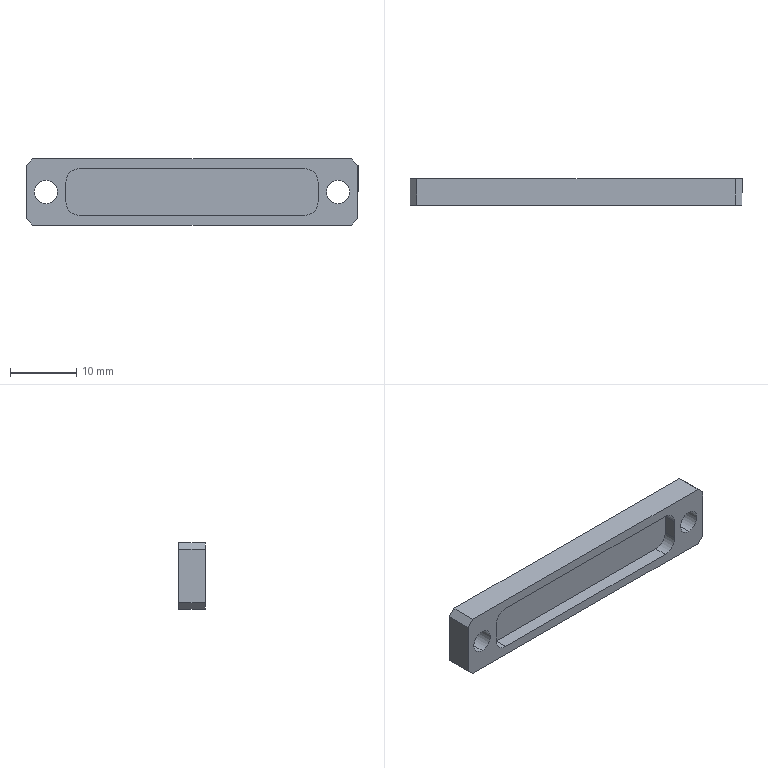Part | SolidWorks | features Chamfer 1, Extrusion 1, HoleWzd 1, ICE 1 | 1 solid | 23 faces | box 50 x 4 x 10 mm | volume 1390 mm3 | plane 15 | cylinder 8 | commonest cylinder face diameters 3.5 x4 4 x4
STEP:
#1=CARTESIAN_POINT('',(-22.,-2.,-1.75));
#2=VERTEX_POINT('',#1);
#3=CARTESIAN_POINT('',(-22.,-2.,1.75));
#4=VERTEX_POINT('',#3);
#5=CARTESIAN_POINT('',(-22.,-2.,0.));
#6=DIRECTION('',(0.,1.,0.));
#7=DIRECTION('',(0.,0.,1.));
#8=AXIS2_PLACEMENT_3D('',#5,#6,#7);
#9=CIRCLE('',#8,1.75);
#10=EDGE_CURVE('',#2,#4,#9,.T.);
#11=ORIENTED_EDGE('',*,*,#10,.F.);
#12=CARTESIAN_POINT('',(-22.,2.,-1.75));
#13=VERTEX_POINT('',#12);
#14=CARTESIAN_POINT('',(-22.,2.,-1.75));
#15=DIRECTION('',(0.,1.,0.));
#16=VECTOR('',#15,1000.);
#17=LINE('',#14,#16);
#18=EDGE_CURVE('',#2,#13,#17,.T.);
#19=ORIENTED_EDGE('',*,*,#18,.T.);
#20=CARTESIAN_POINT('',(-22.,2.,1.75));
#21=VERTEX_POINT('',#20);
#22=CARTESIAN_POINT('',(-22.,2.,0.));
#23=DIRECTION('',(0.,1.,0.));
#24=DIRECTION('',(0.,0.,1.));
#25=AXIS2_PLACEMENT_3D('',#22,#23,#24);
#26=CIRCLE('',#25,1.75);
#27=EDGE_CURVE('',#13,#21,#26,.T.);
#28=ORIENTED_EDGE('',*,*,#27,.T.);
#29=CARTESIAN_POINT('',(-22.,2.,1.75));
#30=DIRECTION('',(0.,1.,0.));
#31=VECTOR('',#30,1000.);
#32=LINE('',#29,#31);
#33=EDGE_CURVE('',#4,#21,#32,.T.);
#34=ORIENTED_EDGE('',*,*,#33,.F.);
#35=EDGE_LOOP('',(#11,#19,#28,#34));
#36=FACE_OUTER_BOUND('',#35,.T.);
#37=CARTESIAN_POINT('',(-22.,2.,0.));
#38=DIRECTION('',(0.,1.,0.));
#39=DIRECTION('',(0.,0.,1.));
#40=AXIS2_PLACEMENT_3D('',#37,#38,#39);
#41=CYLINDRICAL_SURFACE('',#40,1.75);
#42=ADVANCED_FACE('',(#36),#41,.F.);
#43=CARTESIAN_POINT('',(22.,-2.,-1.75));
#44=VERTEX_POINT('',#43);
#45=CARTESIAN_POINT('',(22.,-2.,1.75));
#46=VERTEX_POINT('',#45);
#47=CARTESIAN_POINT('',(22.,-2.,0.));
#48=DIRECTION('',(0.,1.,0.));
#49=DIRECTION('',(0.,0.,1.));
#50=AXIS2_PLACEMENT_3D('',#47,#48,#49);
#51=CIRCLE('',#50,1.75);
#52=EDGE_CURVE('',#44,#46,#51,.T.);
#53=ORIENTED_EDGE('',*,*,#52,.F.);
#54=CARTESIAN_POINT('',(22.,2.,-1.75));
#55=VERTEX_POINT('',#54);
#56=CARTESIAN_POINT('',(22.,2.,-1.75));
#57=DIRECTION('',(0.,1.,0.));
#58=VECTOR('',#57,1000.);
#59=LINE('',#56,#58);
#60=EDGE_CURVE('',#44,#55,#59,.T.);
#61=ORIENTED_EDGE('',*,*,#60,.T.);
#62=CARTESIAN_POINT('',(22.,2.,1.75));
#63=VERTEX_POINT('',#62);
#64=CARTESIAN_POINT('',(22.,2.,0.));
#65=DIRECTION('',(0.,1.,0.));
#66=DIRECTION('',(0.,0.,1.));
#67=AXIS2_PLACEMENT_3D('',#64,#65,#66);
#68=CIRCLE('',#67,1.75);
#69=EDGE_CURVE('',#55,#63,#68,.T.);
#70=ORIENTED_EDGE('',*,*,#69,.T.);
#71=CARTESIAN_POINT('',(22.,2.,1.75));
#72=DIRECTION('',(0.,1.,0.));
#73=VECTOR('',#72,1000.);
#74=LINE('',#71,#73);
#75=EDGE_CURVE('',#46,#63,#74,.T.);
#76=ORIENTED_EDGE('',*,*,#75,.F.);
#77=EDGE_LOOP('',(#53,#61,#70,#76));
#78=FACE_OUTER_BOUND('',#77,.T.);
#79=CARTESIAN_POINT('',(22.,2.,0.));
#80=DIRECTION('',(0.,1.,0.));
#81=DIRECTION('',(0.,0.,1.));
#82=AXIS2_PLACEMENT_3D('',#79,#80,#81);
#83=CYLINDRICAL_SURFACE('',#82,1.75);
#84=ADVANCED_FACE('',(#78),#83,.F.);
#85=CARTESIAN_POINT('',(25.,-2.,4.));
#86=VERTEX_POINT('',#85);
#87=CARTESIAN_POINT('',(25.,-2.,-4.));
#88=VERTEX_POINT('',#87);
#89=CARTESIAN_POINT('',(25.,-2.,-5.));
#90=DIRECTION('',(0.,0.,-1.));
#91=VECTOR('',#90,1000.);
#92=LINE('',#89,#91);
#93=EDGE_CURVE('',#86,#88,#92,.T.);
#94=ORIENTED_EDGE('',*,*,#93,.T.);
#95=CARTESIAN_POINT('',(25.,2.,-4.));
#96=VERTEX_POINT('',#95);
#97=CARTESIAN_POINT('',(25.,2.,-4.));
#98=DIRECTION('',(0.,1.,0.));
#99=VECTOR('',#98,1000.);
#100=LINE('',#97,#99);
#101=EDGE_CURVE('',#88,#96,#100,.T.);
#102=ORIENTED_EDGE('',*,*,#101,.T.);
#103=CARTESIAN_POINT('',(25.,2.,4.));
#104=VERTEX_POINT('',#103);
#105=CARTESIAN_POINT('',(25.,2.,-5.));
#106=DIRECTION('',(0.,0.,-1.));
#107=VECTOR('',#106,1000.);
#108=LINE('',#105,#107);
#109=EDGE_CURVE('',#104,#96,#108,.T.);
#110=ORIENTED_EDGE('',*,*,#109,.F.);
#111=CARTESIAN_POINT('',(25.,2.,4.));
#112=DIRECTION('',(0.,-1.,0.));
#113=VECTOR('',#112,1000.);
#114=LINE('',#111,#113);
#115=EDGE_CURVE('',#104,#86,#114,.T.);
#116=ORIENTED_EDGE('',*,*,#115,.T.);
#117=EDGE_LOOP('',(#94,#102,#110,#116));
#118=FACE_OUTER_BOUND('',#117,.T.);
#119=CARTESIAN_POINT('',(25.,2.,-5.));
#120=DIRECTION('',(-1.,0.,0.));
#121=DIRECTION('',(0.,0.,1.));
#122=AXIS2_PLACEMENT_3D('',#119,#120,#121);
#123=PLANE('',#122);
#124=ADVANCED_FACE('',(#118),#123,.F.);
#125=CARTESIAN_POINT('',(24.,2.,-5.));
#126=VERTEX_POINT('',#125);
#127=CARTESIAN_POINT('',(-24.,2.,-5.));
#128=VERTEX_POINT('',#127);
#129=CARTESIAN_POINT('',(-25.,2.,-5.));
#130=DIRECTION('',(-1.,0.,0.));
#131=VECTOR('',#130,1000.);
#132=LINE('',#129,#131);
#133=EDGE_CURVE('',#126,#128,#132,.T.);
#134=ORIENTED_EDGE('',*,*,#133,.F.);
#135=CARTESIAN_POINT('',(24.,-2.,-5.));
#136=VERTEX_POINT('',#135);
#137=CARTESIAN_POINT('',(24.,2.,-5.));
#138=DIRECTION('',(0.,-1.,0.));
#139=VECTOR('',#138,1000.);
#140=LINE('',#137,#139);
#141=EDGE_CURVE('',#126,#136,#140,.T.);
#142=ORIENTED_EDGE('',*,*,#141,.T.);
#143=CARTESIAN_POINT('',(-24.,-2.,-5.));
#144=VERTEX_POINT('',#143);
#145=CARTESIAN_POINT('',(-25.,-2.,-5.));
#146=DIRECTION('',(-1.,0.,0.));
#147=VECTOR('',#146,1000.);
#148=LINE('',#145,#147);
#149=EDGE_CURVE('',#136,#144,#148,.T.);
#150=ORIENTED_EDGE('',*,*,#149,.T.);
#151=CARTESIAN_POINT('',(-24.,2.,-5.));
#152=DIRECTION('',(0.,1.,0.));
#153=VECTOR('',#152,1000.);
#154=LINE('',#151,#153);
#155=EDGE_CURVE('',#144,#128,#154,.T.);
#156=ORIENTED_EDGE('',*,*,#155,.T.);
#157=EDGE_LOOP('',(#134,#142,#150,#156));
#158=FACE_OUTER_BOUND('',#157,.T.);
#159=CARTESIAN_POINT('',(-25.,2.,-5.));
#160=DIRECTION('',(0.,0.,1.));
#161=DIRECTION('',(1.,0.,0.));
#162=AXIS2_PLACEMENT_3D('',#159,#160,#161);
#163=PLANE('',#162);
#164=ADVANCED_FACE('',(#158),#163,.F.);
#165=CARTESIAN_POINT('',(-25.,2.,-4.));
#166=VERTEX_POINT('',#165);
#167=CARTESIAN_POINT('',(-25.,2.,4.));
#168=VERTEX_POINT('',#167);
#169=CARTESIAN_POINT('',(-25.,2.,-5.));
#170=DIRECTION('',(0.,0.,1.));
#171=VECTOR('',#170,1000.);
#172=LINE('',#169,#171);
#173=EDGE_CURVE('',#166,#168,#172,.T.);
#174=ORIENTED_EDGE('',*,*,#173,.F.);
#175=CARTESIAN_POINT('',(-25.,-2.,-4.));
#176=VERTEX_POINT('',#175);
#177=CARTESIAN_POINT('',(-25.,2.,-4.));
#178=DIRECTION('',(0.,-1.,0.));
#179=VECTOR('',#178,1000.);
#180=LINE('',#177,#179);
#181=EDGE_CURVE('',#166,#176,#180,.T.);
#182=ORIENTED_EDGE('',*,*,#181,.T.);
#183=CARTESIAN_POINT('',(-25.,-2.,4.));
#184=VERTEX_POINT('',#183);
#185=CARTESIAN_POINT('',(-25.,-2.,-5.));
#186=DIRECTION('',(0.,0.,1.));
#187=VECTOR('',#186,1000.);
#188=LINE('',#185,#187);
#189=EDGE_CURVE('',#176,#184,#188,.T.);
#190=ORIENTED_EDGE('',*,*,#189,.T.);
#191=CARTESIAN_POINT('',(-25.,2.,4.));
#192=DIRECTION('',(0.,1.,0.));
#193=VECTOR('',#192,1000.);
#194=LINE('',#191,#193);
#195=EDGE_CURVE('',#184,#168,#194,.T.);
#196=ORIENTED_EDGE('',*,*,#195,.T.);
#197=EDGE_LOOP('',(#174,#182,#190,#196));
#198=FACE_OUTER_BOUND('',#197,.T.);
#199=CARTESIAN_POINT('',(-25.,2.,-5.));
#200=DIRECTION('',(1.,0.,0.));
#201=DIRECTION('',(0.,0.,-1.));
#202=AXIS2_PLACEMENT_3D('',#199,#200,#201);
#203=PLANE('',#202);
#204=ADVANCED_FACE('',(#198),#203,.F.);
#205=CARTESIAN_POINT('',(-24.,-2.,5.));
#206=VERTEX_POINT('',#205);
#207=CARTESIAN_POINT('',(24.,-2.,5.));
#208=VERTEX_POINT('',#207);
#209=CARTESIAN_POINT('',(-25.,-2.,5.));
#210=DIRECTION('',(1.,0.,0.));
#211=VECTOR('',#210,1000.);
#212=LINE('',#209,#211);
#213=EDGE_CURVE('',#206,#208,#212,.T.);
#214=ORIENTED_EDGE('',*,*,#213,.T.);
#215=CARTESIAN_POINT('',(24.,2.,5.));
#216=VERTEX_POINT('',#215);
#217=CARTESIAN_POINT('',(24.,2.,5.));
#218=DIRECTION('',(0.,1.,0.));
#219=VECTOR('',#218,1000.);
#220=LINE('',#217,#219);
#221=EDGE_CURVE('',#208,#216,#220,.T.);
#222=ORIENTED_EDGE('',*,*,#221,.T.);
#223=CARTESIAN_POINT('',(-24.,2.,5.));
#224=VERTEX_POINT('',#223);
#225=CARTESIAN_POINT('',(-25.,2.,5.));
#226=DIRECTION('',(1.,0.,0.));
#227=VECTOR('',#226,1000.);
#228=LINE('',#225,#227);
#229=EDGE_CURVE('',#224,#216,#228,.T.);
#230=ORIENTED_EDGE('',*,*,#229,.F.);
#231=CARTESIAN_POINT('',(-24.,2.,5.));
#232=DIRECTION('',(0.,-1.,0.));
#233=VECTOR('',#232,1000.);
#234=LINE('',#231,#233);
#235=EDGE_CURVE('',#224,#206,#234,.T.);
#236=ORIENTED_EDGE('',*,*,#235,.T.);
#237=EDGE_LOOP('',(#214,#222,#230,#236));
#238=FACE_OUTER_BOUND('',#237,.T.);
#239=CARTESIAN_POINT('',(-25.,2.,5.));
#240=DIRECTION('',(0.,0.,-1.));
#241=DIRECTION('',(-1.,0.,0.));
#242=AXIS2_PLACEMENT_3D('',#239,#240,#241);
#243=PLANE('',#242);
#244=ADVANCED_FACE('',(#238),#243,.F.);
#245=CARTESIAN_POINT('',(-22.,2.,0.));
#246=DIRECTION('',(0.,1.,0.));
#247=DIRECTION('',(0.,0.,1.));
#248=AXIS2_PLACEMENT_3D('',#245,#246,#247);
#249=CIRCLE('',#248,1.75);
#250=EDGE_CURVE('',#21,#13,#249,.T.);
#251=ORIENTED_EDGE('',*,*,#250,.F.);
#252=ORIENTED_EDGE('',*,*,#27,.F.);
#253=EDGE_LOOP('',(#251,#252));
#254=FACE_BOUND('',#253,.T.);
#255=CARTESIAN_POINT('',(22.,2.,0.));
#256=DIRECTION('',(0.,1.,0.));
#257=DIRECTION('',(0.,0.,1.));
#258=AXIS2_PLACEMENT_3D('',#255,#256,#257);
#259=CIRCLE('',#258,1.75);
#260=EDGE_CURVE('',#63,#55,#259,.T.);
#261=ORIENTED_EDGE('',*,*,#260,.F.);
#262=ORIENTED_EDGE('',*,*,#69,.F.);
#263=EDGE_LOOP('',(#261,#262));
#264=FACE_BOUND('',#263,.T.);
#265=ORIENTED_EDGE('',*,*,#109,.T.);
#266=CARTESIAN_POINT('',(14.5,2.,-14.5));
#267=DIRECTION('',(-0.7071,0.,-0.7071));
#268=VECTOR('',#267,1000.);
#269=LINE('',#266,#268);
#270=EDGE_CURVE('',#96,#126,#269,.T.);
#271=ORIENTED_EDGE('',*,*,#270,.T.);
#272=ORIENTED_EDGE('',*,*,#133,.T.);
#273=CARTESIAN_POINT('',(-14.5,2.,-14.5));
#274=DIRECTION('',(-0.7071,0.,0.7071));
#275=VECTOR('',#274,1000.);
#276=LINE('',#273,#275);
#277=EDGE_CURVE('',#128,#166,#276,.T.);
#278=ORIENTED_EDGE('',*,*,#277,.T.);
#279=ORIENTED_EDGE('',*,*,#173,.T.);
#280=CARTESIAN_POINT('',(-14.5,2.,14.5));
#281=DIRECTION('',(0.7071,0.,0.7071));
#282=VECTOR('',#281,1000.);
#283=LINE('',#280,#282);
#284=EDGE_CURVE('',#168,#224,#283,.T.);
#285=ORIENTED_EDGE('',*,*,#284,.T.);
#286=ORIENTED_EDGE('',*,*,#229,.T.);
#287=CARTESIAN_POINT('',(14.5,2.,14.5));
#288=DIRECTION('',(0.7071,0.,-0.7071));
#289=VECTOR('',#288,1000.);
#290=LINE('',#287,#289);
#291=EDGE_CURVE('',#216,#104,#290,.T.);
#292=ORIENTED_EDGE('',*,*,#291,.T.);
#293=EDGE_LOOP('',(#265,#271,#272,#278,#279,#285,#286,#292));
#294=FACE_OUTER_BOUND('',#293,.T.);
#295=CARTESIAN_POINT('',(0.,2.,0.));
#296=DIRECTION('',(0.,1.,0.));
#297=DIRECTION('',(0.,0.,1.));
#298=AXIS2_PLACEMENT_3D('',#295,#296,#297);
#299=PLANE('',#298);
#300=ADVANCED_FACE('',(#254,#264,#294),#299,.T.);
#301=CARTESIAN_POINT('',(17.,-2.,3.5));
#302=VERTEX_POINT('',#301);
#303=CARTESIAN_POINT('',(-17.,-2.,3.5));
#304=VERTEX_POINT('',#303);
#305=CARTESIAN_POINT('',(-17.,-2.,3.5));
#306=DIRECTION('',(-1.,0.,0.));
#307=VECTOR('',#306,1000.);
#308=LINE('',#305,#307);
#309=EDGE_CURVE('',#302,#304,#308,.T.);
#310=ORIENTED_EDGE('',*,*,#309,.F.);
#311=CARTESIAN_POINT('',(19.,-2.,1.5));
#312=VERTEX_POINT('',#311);
#313=CARTESIAN_POINT('',(17.,-2.,1.5));
#314=DIRECTION('',(0.,-1.,0.));
#315=DIRECTION('',(0.,0.,1.));
#316=AXIS2_PLACEMENT_3D('',#313,#314,#315);
#317=CIRCLE('',#316,2.);
#318=EDGE_CURVE('',#312,#302,#317,.T.);
#319=ORIENTED_EDGE('',*,*,#318,.F.);
#320=CARTESIAN_POINT('',(19.,-2.,-1.5));
#321=VERTEX_POINT('',#320);
#322=CARTESIAN_POINT('',(19.,-2.,1.5));
#323=DIRECTION('',(0.,0.,1.));
#324=VECTOR('',#323,1000.);
#325=LINE('',#322,#324);
#326=EDGE_CURVE('',#321,#312,#325,.T.);
#327=ORIENTED_EDGE('',*,*,#326,.F.);
#328=CARTESIAN_POINT('',(17.,-2.,-3.5));
#329=VERTEX_POINT('',#328);
#330=CARTESIAN_POINT('',(17.,-2.,-1.5));
#331=DIRECTION('',(0.,-1.,0.));
#332=DIRECTION('',(0.,0.,1.));
#333=AXIS2_PLACEMENT_3D('',#330,#331,#332);
#334=CIRCLE('',#333,2.);
#335=EDGE_CURVE('',#329,#321,#334,.T.);
#336=ORIENTED_EDGE('',*,*,#335,.F.);
#337=CARTESIAN_POINT('',(-17.,-2.,-3.5));
#338=VERTEX_POINT('',#337);
#339=CARTESIAN_POINT('',(-17.,-2.,-3.5));
#340=DIRECTION('',(1.,0.,0.));
#341=VECTOR('',#340,1000.);
#342=LINE('',#339,#341);
#343=EDGE_CURVE('',#338,#329,#342,.T.);
#344=ORIENTED_EDGE('',*,*,#343,.F.);
#345=CARTESIAN_POINT('',(-19.,-2.,-1.5));
#346=VERTEX_POINT('',#345);
#347=CARTESIAN_POINT('',(-17.,-2.,-1.5));
#348=DIRECTION('',(0.,-1.,0.));
#349=DIRECTION('',(0.,0.,1.));
#350=AXIS2_PLACEMENT_3D('',#347,#348,#349);
#351=CIRCLE('',#350,2.);
#352=EDGE_CURVE('',#346,#338,#351,.T.);
#353=ORIENTED_EDGE('',*,*,#352,.F.);
#354=CARTESIAN_POINT('',(-19.,-2.,1.5));
#355=VERTEX_POINT('',#354);
#356=CARTESIAN_POINT('',(-19.,-2.,1.5));
#357=DIRECTION('',(0.,0.,-1.));
#358=VECTOR('',#357,1000.);
#359=LINE('',#356,#358);
#360=EDGE_CURVE('',#355,#346,#359,.T.);
#361=ORIENTED_EDGE('',*,*,#360,.F.);
#362=CARTESIAN_POINT('',(-17.,-2.,1.5));
#363=DIRECTION('',(0.,-1.,0.));
#364=DIRECTION('',(0.,0.,-1.));
#365=AXIS2_PLACEMENT_3D('',#362,#363,#364);
#366=CIRCLE('',#365,2.);
#367=EDGE_CURVE('',#304,#355,#366,.T.);
#368=ORIENTED_EDGE('',*,*,#367,.F.);
#369=EDGE_LOOP('',(#310,#319,#327,#336,#344,#353,#361,#368));
#370=FACE_BOUND('',#369,.T.);
#371=CARTESIAN_POINT('',(-22.,-2.,0.));
#372=DIRECTION('',(0.,1.,0.));
#373=DIRECTION('',(0.,0.,1.));
#374=AXIS2_PLACEMENT_3D('',#371,#372,#373);
#375=CIRCLE('',#374,1.75);
#376=EDGE_CURVE('',#4,#2,#375,.T.);
#377=ORIENTED_EDGE('',*,*,#376,.T.);
#378=ORIENTED_EDGE('',*,*,#10,.T.);
#379=EDGE_LOOP('',(#377,#378));
#380=FACE_BOUND('',#379,.T.);
#381=CARTESIAN_POINT('',(22.,-2.,0.));
#382=DIRECTION('',(0.,1.,0.));
#383=DIRECTION('',(0.,0.,1.));
#384=AXIS2_PLACEMENT_3D('',#381,#382,#383);
#385=CIRCLE('',#384,1.75);
#386=EDGE_CURVE('',#46,#44,#385,.T.);
#387=ORIENTED_EDGE('',*,*,#386,.T.);
#388=ORIENTED_EDGE('',*,*,#52,.T.);
#389=EDGE_LOOP('',(#387,#388));
#390=FACE_BOUND('',#389,.T.);
#391=ORIENTED_EDGE('',*,*,#149,.F.);
#392=CARTESIAN_POINT('',(24.,-2.,-5.));
#393=DIRECTION('',(0.7071,0.,0.7071));
#394=VECTOR('',#393,1000.);
#395=LINE('',#392,#394);
#396=EDGE_CURVE('',#136,#88,#395,.T.);
#397=ORIENTED_EDGE('',*,*,#396,.T.);
#398=ORIENTED_EDGE('',*,*,#93,.F.);
#399=CARTESIAN_POINT('',(25.,-2.,4.));
#400=DIRECTION('',(-0.7071,0.,0.7071));
#401=VECTOR('',#400,1000.);
#402=LINE('',#399,#401);
#403=EDGE_CURVE('',#86,#208,#402,.T.);
#404=ORIENTED_EDGE('',*,*,#403,.T.);
#405=ORIENTED_EDGE('',*,*,#213,.F.);
#406=CARTESIAN_POINT('',(-24.,-2.,5.));
#407=DIRECTION('',(-0.7071,0.,-0.7071));
#408=VECTOR('',#407,1000.);
#409=LINE('',#406,#408);
#410=EDGE_CURVE('',#206,#184,#409,.T.);
#411=ORIENTED_EDGE('',*,*,#410,.T.);
#412=ORIENTED_EDGE('',*,*,#189,.F.);
#413=CARTESIAN_POINT('',(-25.,-2.,-4.));
#414=DIRECTION('',(0.7071,0.,-0.7071));
#415=VECTOR('',#414,1000.);
#416=LINE('',#413,#415);
#417=EDGE_CURVE('',#176,#144,#416,.T.);
#418=ORIENTED_EDGE('',*,*,#417,.T.);
#419=EDGE_LOOP('',(#391,#397,#398,#404,#405,#411,#412,#418));
#420=FACE_OUTER_BOUND('',#419,.T.);
#421=CARTESIAN_POINT('',(0.,-2.,0.));
#422=DIRECTION('',(0.,1.,0.));
#423=DIRECTION('',(0.,0.,1.));
#424=AXIS2_PLACEMENT_3D('',#421,#422,#423);
#425=PLANE('',#424);
#426=ADVANCED_FACE('',(#370,#380,#390,#420),#425,.F.);
#427=ORIENTED_EDGE('',*,*,#60,.F.);
#428=ORIENTED_EDGE('',*,*,#386,.F.);
#429=ORIENTED_EDGE('',*,*,#75,.T.);
#430=ORIENTED_EDGE('',*,*,#260,.T.);
#431=EDGE_LOOP('',(#427,#428,#429,#430));
#432=FACE_OUTER_BOUND('',#431,.T.);
#433=CARTESIAN_POINT('',(22.,2.,0.));
#434=DIRECTION('',(0.,1.,0.));
#435=DIRECTION('',(0.,0.,1.));
#436=AXIS2_PLACEMENT_3D('',#433,#434,#435);
#437=CYLINDRICAL_SURFACE('',#436,1.75);
#438=ADVANCED_FACE('',(#432),#437,.F.);
#439=ORIENTED_EDGE('',*,*,#18,.F.);
#440=ORIENTED_EDGE('',*,*,#376,.F.);
#441=ORIENTED_EDGE('',*,*,#33,.T.);
#442=ORIENTED_EDGE('',*,*,#250,.T.);
#443=EDGE_LOOP('',(#439,#440,#441,#442));
#444=FACE_OUTER_BOUND('',#443,.T.);
#445=CARTESIAN_POINT('',(-22.,2.,0.));
#446=DIRECTION('',(0.,1.,0.));
#447=DIRECTION('',(0.,0.,1.));
#448=AXIS2_PLACEMENT_3D('',#445,#446,#447);
#449=CYLINDRICAL_SURFACE('',#448,1.75);
#450=ADVANCED_FACE('',(#444),#449,.F.);
#451=ORIENTED_EDGE('',*,*,#270,.F.);
#452=ORIENTED_EDGE('',*,*,#101,.F.);
#453=ORIENTED_EDGE('',*,*,#396,.F.);
#454=ORIENTED_EDGE('',*,*,#141,.F.);
#455=EDGE_LOOP('',(#451,#452,#453,#454));
#456=FACE_OUTER_BOUND('',#455,.T.);
#457=CARTESIAN_POINT('',(24.,2.,-5.));
#458=DIRECTION('',(-0.7071,0.,0.7071));
#459=DIRECTION('',(0.,-1.,0.));
#460=AXIS2_PLACEMENT_3D('',#457,#458,#459);
#461=PLANE('',#460);
#462=ADVANCED_FACE('',(#456),#461,.F.);
#463=ORIENTED_EDGE('',*,*,#291,.F.);
#464=ORIENTED_EDGE('',*,*,#221,.F.);
#465=ORIENTED_EDGE('',*,*,#403,.F.);
#466=ORIENTED_EDGE('',*,*,#115,.F.);
#467=EDGE_LOOP('',(#463,#464,#465,#466));
#468=FACE_OUTER_BOUND('',#467,.T.);
#469=CARTESIAN_POINT('',(25.,2.,4.));
#470=DIRECTION('',(-0.7071,0.,-0.7071));
#471=DIRECTION('',(0.,-1.,0.));
#472=AXIS2_PLACEMENT_3D('',#469,#470,#471);
#473=PLANE('',#472);
#474=ADVANCED_FACE('',(#468),#473,.F.);
#475=ORIENTED_EDGE('',*,*,#277,.F.);
#476=ORIENTED_EDGE('',*,*,#155,.F.);
#477=ORIENTED_EDGE('',*,*,#417,.F.);
#478=ORIENTED_EDGE('',*,*,#181,.F.);
#479=EDGE_LOOP('',(#475,#476,#477,#478));
#480=FACE_OUTER_BOUND('',#479,.T.);
#481=CARTESIAN_POINT('',(-25.,2.,-4.));
#482=DIRECTION('',(0.7071,0.,0.7071));
#483=DIRECTION('',(0.,-1.,0.));
#484=AXIS2_PLACEMENT_3D('',#481,#482,#483);
#485=PLANE('',#484);
#486=ADVANCED_FACE('',(#480),#485,.F.);
#487=ORIENTED_EDGE('',*,*,#284,.F.);
#488=ORIENTED_EDGE('',*,*,#195,.F.);
#489=ORIENTED_EDGE('',*,*,#410,.F.);
#490=ORIENTED_EDGE('',*,*,#235,.F.);
#491=EDGE_LOOP('',(#487,#488,#489,#490));
#492=FACE_OUTER_BOUND('',#491,.T.);
#493=CARTESIAN_POINT('',(-24.,2.,5.));
#494=DIRECTION('',(0.7071,0.,-0.7071));
#495=DIRECTION('',(0.,-1.,0.));
#496=AXIS2_PLACEMENT_3D('',#493,#494,#495);
#497=PLANE('',#496);
#498=ADVANCED_FACE('',(#492),#497,.F.);
#499=ORIENTED_EDGE('',*,*,#318,.T.);
#500=CARTESIAN_POINT('',(17.,0.,3.5));
#501=VERTEX_POINT('',#500);
#502=CARTESIAN_POINT('',(17.,0.,3.5));
#503=DIRECTION('',(0.,-1.,0.));
#504=VECTOR('',#503,1000.);
#505=LINE('',#502,#504);
#506=EDGE_CURVE('',#501,#302,#505,.T.);
#507=ORIENTED_EDGE('',*,*,#506,.F.);
#508=CARTESIAN_POINT('',(19.,0.,1.5));
#509=VERTEX_POINT('',#508);
#510=CARTESIAN_POINT('',(17.,0.,1.5));
#511=DIRECTION('',(0.,-1.,0.));
#512=DIRECTION('',(0.,0.,1.));
#513=AXIS2_PLACEMENT_3D('',#510,#511,#512);
#514=CIRCLE('',#513,2.);
#515=EDGE_CURVE('',#509,#501,#514,.T.);
#516=ORIENTED_EDGE('',*,*,#515,.F.);
#517=CARTESIAN_POINT('',(19.,0.,1.5));
#518=DIRECTION('',(0.,-1.,0.));
#519=VECTOR('',#518,1000.);
#520=LINE('',#517,#519);
#521=EDGE_CURVE('',#509,#312,#520,.T.);
#522=ORIENTED_EDGE('',*,*,#521,.T.);
#523=EDGE_LOOP('',(#499,#507,#516,#522));
#524=FACE_OUTER_BOUND('',#523,.T.);
#525=CARTESIAN_POINT('',(17.,0.,1.5));
#526=DIRECTION('',(0.,-1.,0.));
#527=DIRECTION('',(0.,0.,-1.));
#528=AXIS2_PLACEMENT_3D('',#525,#526,#527);
#529=CYLINDRICAL_SURFACE('',#528,2.);
#530=ADVANCED_FACE('',(#524),#529,.F.);
#531=ORIENTED_EDGE('',*,*,#326,.T.);
#532=ORIENTED_EDGE('',*,*,#521,.F.);
#533=CARTESIAN_POINT('',(19.,0.,-1.5));
#534=VERTEX_POINT('',#533);
#535=CARTESIAN_POINT('',(19.,0.,1.5));
#536=DIRECTION('',(0.,0.,1.));
#537=VECTOR('',#536,1000.);
#538=LINE('',#535,#537);
#539=EDGE_CURVE('',#534,#509,#538,.T.);
#540=ORIENTED_EDGE('',*,*,#539,.F.);
#541=CARTESIAN_POINT('',(19.,0.,-1.5));
#542=DIRECTION('',(0.,-1.,0.));
#543=VECTOR('',#542,1000.);
#544=LINE('',#541,#543);
#545=EDGE_CURVE('',#534,#321,#544,.T.);
#546=ORIENTED_EDGE('',*,*,#545,.T.);
#547=EDGE_LOOP('',(#531,#532,#540,#546));
#548=FACE_OUTER_BOUND('',#547,.T.);
#549=CARTESIAN_POINT('',(19.,0.,1.5));
#550=DIRECTION('',(1.,0.,0.));
#551=DIRECTION('',(0.,0.,-1.));
#552=AXIS2_PLACEMENT_3D('',#549,#550,#551);
#553=PLANE('',#552);
#554=ADVANCED_FACE('',(#548),#553,.F.);
#555=ORIENTED_EDGE('',*,*,#335,.T.);
#556=ORIENTED_EDGE('',*,*,#545,.F.);
#557=CARTESIAN_POINT('',(17.,0.,-3.5));
#558=VERTEX_POINT('',#557);
#559=CARTESIAN_POINT('',(17.,0.,-1.5));
#560=DIRECTION('',(0.,-1.,0.));
#561=DIRECTION('',(0.,0.,1.));
#562=AXIS2_PLACEMENT_3D('',#559,#560,#561);
#563=CIRCLE('',#562,2.);
#564=EDGE_CURVE('',#558,#534,#563,.T.);
#565=ORIENTED_EDGE('',*,*,#564,.F.);
#566=CARTESIAN_POINT('',(17.,0.,-3.5));
#567=DIRECTION('',(0.,-1.,0.));
#568=VECTOR('',#567,1000.);
#569=LINE('',#566,#568);
#570=EDGE_CURVE('',#558,#329,#569,.T.);
#571=ORIENTED_EDGE('',*,*,#570,.T.);
#572=EDGE_LOOP('',(#555,#556,#565,#571));
#573=FACE_OUTER_BOUND('',#572,.T.);
#574=CARTESIAN_POINT('',(17.,0.,-1.5));
#575=DIRECTION('',(0.,-1.,0.));
#576=DIRECTION('',(0.,0.,-1.));
#577=AXIS2_PLACEMENT_3D('',#574,#575,#576);
#578=CYLINDRICAL_SURFACE('',#577,2.);
#579=ADVANCED_FACE('',(#573),#578,.F.);
#580=ORIENTED_EDGE('',*,*,#343,.T.);
#581=ORIENTED_EDGE('',*,*,#570,.F.);
#582=CARTESIAN_POINT('',(-17.,0.,-3.5));
#583=VERTEX_POINT('',#582);
#584=CARTESIAN_POINT('',(-17.,0.,-3.5));
#585=DIRECTION('',(1.,0.,0.));
#586=VECTOR('',#585,1000.);
#587=LINE('',#584,#586);
#588=EDGE_CURVE('',#583,#558,#587,.T.);
#589=ORIENTED_EDGE('',*,*,#588,.F.);
#590=CARTESIAN_POINT('',(-17.,0.,-3.5));
#591=DIRECTION('',(0.,-1.,0.));
#592=VECTOR('',#591,1000.);
#593=LINE('',#590,#592);
#594=EDGE_CURVE('',#583,#338,#593,.T.);
#595=ORIENTED_EDGE('',*,*,#594,.T.);
#596=EDGE_LOOP('',(#580,#581,#589,#595));
#597=FACE_OUTER_BOUND('',#596,.T.);
#598=CARTESIAN_POINT('',(-17.,0.,-3.5));
#599=DIRECTION('',(0.,0.,-1.));
#600=DIRECTION('',(-1.,0.,0.));
#601=AXIS2_PLACEMENT_3D('',#598,#599,#600);
#602=PLANE('',#601);
#603=ADVANCED_FACE('',(#597),#602,.F.);
#604=ORIENTED_EDGE('',*,*,#352,.T.);
#605=ORIENTED_EDGE('',*,*,#594,.F.);
#606=CARTESIAN_POINT('',(-19.,0.,-1.5));
#607=VERTEX_POINT('',#606);
#608=CARTESIAN_POINT('',(-17.,0.,-1.5));
#609=DIRECTION('',(0.,-1.,0.));
#610=DIRECTION('',(0.,0.,1.));
#611=AXIS2_PLACEMENT_3D('',#608,#609,#610);
#612=CIRCLE('',#611,2.);
#613=EDGE_CURVE('',#607,#583,#612,.T.);
#614=ORIENTED_EDGE('',*,*,#613,.F.);
#615=CARTESIAN_POINT('',(-19.,0.,-1.5));
#616=DIRECTION('',(0.,-1.,0.));
#617=VECTOR('',#616,1000.);
#618=LINE('',#615,#617);
#619=EDGE_CURVE('',#607,#346,#618,.T.);
#620=ORIENTED_EDGE('',*,*,#619,.T.);
#621=EDGE_LOOP('',(#604,#605,#614,#620));
#622=FACE_OUTER_BOUND('',#621,.T.);
#623=CARTESIAN_POINT('',(-17.,0.,-1.5));
#624=DIRECTION('',(0.,-1.,0.));
#625=DIRECTION('',(0.,0.,-1.));
#626=AXIS2_PLACEMENT_3D('',#623,#624,#625);
#627=CYLINDRICAL_SURFACE('',#626,2.);
#628=ADVANCED_FACE('',(#622),#627,.F.);
#629=ORIENTED_EDGE('',*,*,#360,.T.);
#630=ORIENTED_EDGE('',*,*,#619,.F.);
#631=CARTESIAN_POINT('',(-19.,0.,1.5));
#632=VERTEX_POINT('',#631);
#633=CARTESIAN_POINT('',(-19.,0.,1.5));
#634=DIRECTION('',(0.,0.,-1.));
#635=VECTOR('',#634,1000.);
#636=LINE('',#633,#635);
#637=EDGE_CURVE('',#632,#607,#636,.T.);
#638=ORIENTED_EDGE('',*,*,#637,.F.);
#639=CARTESIAN_POINT('',(-19.,0.,1.5));
#640=DIRECTION('',(0.,-1.,0.));
#641=VECTOR('',#640,1000.);
#642=LINE('',#639,#641);
#643=EDGE_CURVE('',#632,#355,#642,.T.);
#644=ORIENTED_EDGE('',*,*,#643,.T.);
#645=EDGE_LOOP('',(#629,#630,#638,#644));
#646=FACE_OUTER_BOUND('',#645,.T.);
#647=CARTESIAN_POINT('',(-19.,0.,1.5));
#648=DIRECTION('',(-1.,0.,0.));
#649=DIRECTION('',(0.,0.,1.));
#650=AXIS2_PLACEMENT_3D('',#647,#648,#649);
#651=PLANE('',#650);
#652=ADVANCED_FACE('',(#646),#651,.F.);
#653=ORIENTED_EDGE('',*,*,#367,.T.);
#654=ORIENTED_EDGE('',*,*,#643,.F.);
#655=CARTESIAN_POINT('',(-17.,0.,3.5));
#656=VERTEX_POINT('',#655);
#657=CARTESIAN_POINT('',(-17.,0.,1.5));
#658=DIRECTION('',(0.,-1.,0.));
#659=DIRECTION('',(0.,0.,-1.));
#660=AXIS2_PLACEMENT_3D('',#657,#658,#659);
#661=CIRCLE('',#660,2.);
#662=EDGE_CURVE('',#656,#632,#661,.T.);
#663=ORIENTED_EDGE('',*,*,#662,.F.);
#664=CARTESIAN_POINT('',(-17.,0.,3.5));
#665=DIRECTION('',(0.,-1.,0.));
#666=VECTOR('',#665,1000.);
#667=LINE('',#664,#666);
#668=EDGE_CURVE('',#656,#304,#667,.T.);
#669=ORIENTED_EDGE('',*,*,#668,.T.);
#670=EDGE_LOOP('',(#653,#654,#663,#669));
#671=FACE_OUTER_BOUND('',#670,.T.);
#672=CARTESIAN_POINT('',(-17.,0.,1.5));
#673=DIRECTION('',(0.,-1.,0.));
#674=DIRECTION('',(0.,0.,-1.));
#675=AXIS2_PLACEMENT_3D('',#672,#673,#674);
#676=CYLINDRICAL_SURFACE('',#675,2.);
#677=ADVANCED_FACE('',(#671),#676,.F.);
#678=ORIENTED_EDGE('',*,*,#309,.T.);
#679=ORIENTED_EDGE('',*,*,#668,.F.);
#680=CARTESIAN_POINT('',(-17.,0.,3.5));
#681=DIRECTION('',(-1.,0.,0.));
#682=VECTOR('',#681,1000.);
#683=LINE('',#680,#682);
#684=EDGE_CURVE('',#501,#656,#683,.T.);
#685=ORIENTED_EDGE('',*,*,#684,.F.);
#686=ORIENTED_EDGE('',*,*,#506,.T.);
#687=EDGE_LOOP('',(#678,#679,#685,#686));
#688=FACE_OUTER_BOUND('',#687,.T.);
#689=CARTESIAN_POINT('',(-17.,0.,3.5));
#690=DIRECTION('',(0.,0.,1.));
#691=DIRECTION('',(1.,0.,0.));
#692=AXIS2_PLACEMENT_3D('',#689,#690,#691);
#693=PLANE('',#692);
#694=ADVANCED_FACE('',(#688),#693,.F.);
#695=ORIENTED_EDGE('',*,*,#515,.T.);
#696=ORIENTED_EDGE('',*,*,#684,.T.);
#697=ORIENTED_EDGE('',*,*,#662,.T.);
#698=ORIENTED_EDGE('',*,*,#637,.T.);
#699=ORIENTED_EDGE('',*,*,#613,.T.);
#700=ORIENTED_EDGE('',*,*,#588,.T.);
#701=ORIENTED_EDGE('',*,*,#564,.T.);
#702=ORIENTED_EDGE('',*,*,#539,.T.);
#703=EDGE_LOOP('',(#695,#696,#697,#698,#699,#700,#701,#702));
#704=FACE_OUTER_BOUND('',#703,.T.);
#705=CARTESIAN_POINT('',(17.,0.,1.5));
#706=DIRECTION('',(0.,1.,0.));
#707=DIRECTION('',(0.,0.,1.));
#708=AXIS2_PLACEMENT_3D('',#705,#706,#707);
#709=PLANE('',#708);
#710=ADVANCED_FACE('',(#704),#709,.F.);
#711=CLOSED_SHELL('',(#42,#84,#124,#164,#204,#244,#300,#426,#438,#450,#462,#474,#486,#498,#530,#554,#579,#603,#628,#652,#677,#694,#710));
#712=MANIFOLD_SOLID_BREP('',#711);
#713=CARTESIAN_POINT('',(0.,0.,0.));
#714=DIRECTION('',(0.,0.,1.));
#715=DIRECTION('',(1.,0.,0.));
#716=AXIS2_PLACEMENT_3D('',#713,#714,#715);
#717=(LENGTH_UNIT()NAMED_UNIT(*)SI_UNIT(.MILLI.,.METRE.));
#718=UNCERTAINTY_MEASURE_WITH_UNIT(LENGTH_MEASURE(0.00001),#717,'','');
#719=(NAMED_UNIT(*)PLANE_ANGLE_UNIT()SI_UNIT($,.RADIAN.));
#720=(NAMED_UNIT(*)SI_UNIT($,.STERADIAN.)SOLID_ANGLE_UNIT());
#721=(GEOMETRIC_REPRESENTATION_CONTEXT(3)GLOBAL_UNCERTAINTY_ASSIGNED_CONTEXT((#718))GLOBAL_UNIT_ASSIGNED_CONTEXT((#717,#719,#720))REPRESENTATION_CONTEXT('',''));
#722=ADVANCED_BREP_SHAPE_REPRESENTATION('',(#712,#716),#721);